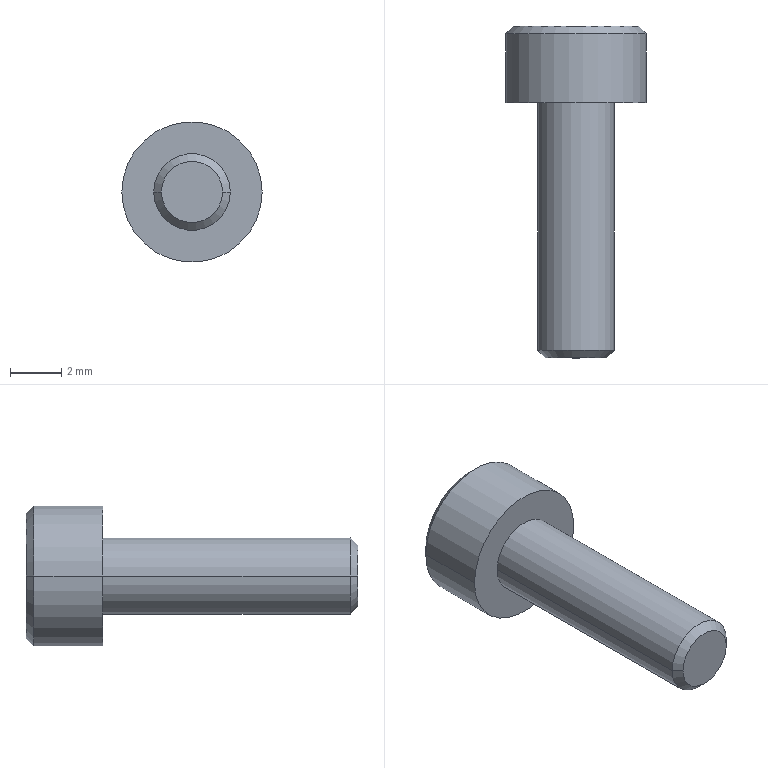Part | NX | 1 solid | 97 faces | box 5.5 x 13 x 5.5 mm | volume 131.454 mm3 | plane 87 | cone 6 | cylinder 4 | commonest cylinder face diameters 3 x2 5.5 x2